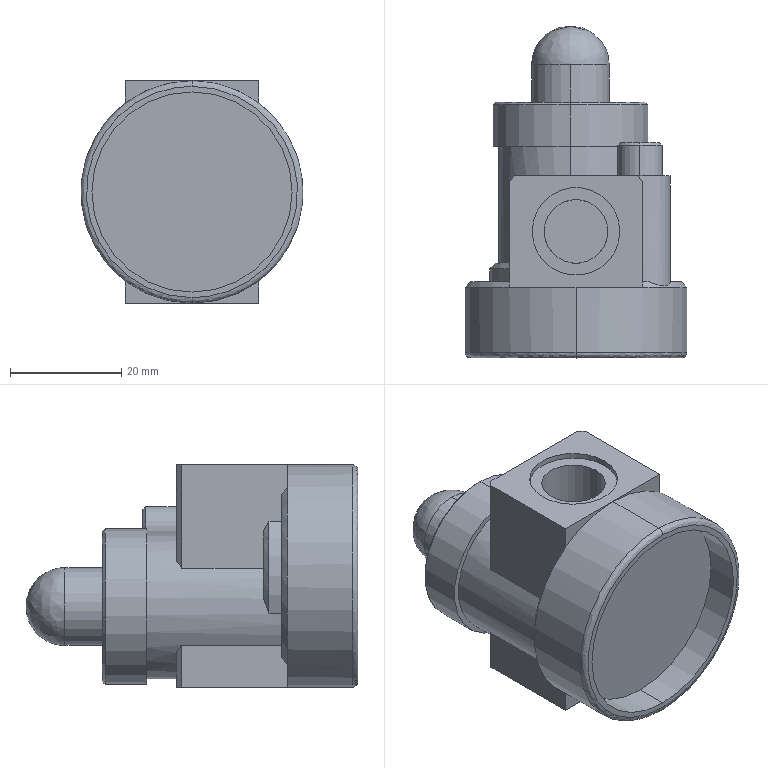Part | SolidWorks | features BaseBody 1 | 1 solid | 72 faces | box 40 x 59.7 x 40 mm | volume 38518 mm3 | plane 33 | cylinder 25 | cone 11 | spline 3 | commonest cylinder face diameters 11.445 x4 15.788 x4 10.95 x3 8 x2 14 x2 26 x2